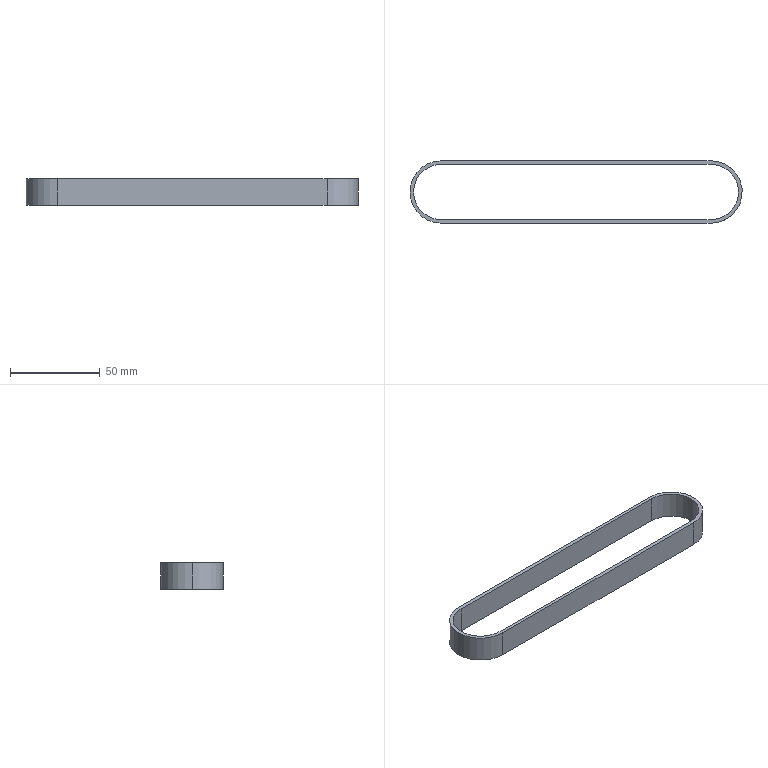Part | STEP file | HTBN400S5M-150 | 1 solid | 12 faces | box 185.61 x 34.88 x 15 mm | volume 12143 mm3 | cylinder 6 | plane 6 | commonest cylinder face diameters 30.88 x3 34.88 x3
STEP:
#1=CARTESIAN_POINT('',(0.,0.,0.));
#2=DIRECTION('',(0.,0.,1.));
#3=DIRECTION('',(1.,0.,0.));
#4=AXIS2_PLACEMENT_3D('',#1,#2,#3);
#5=CARTESIAN_POINT('',(-52.748,15.44,15.));
#6=VERTEX_POINT('',#5);
#7=CARTESIAN_POINT('',(-52.748,15.44,0.));
#8=VERTEX_POINT('',#7);
#9=CARTESIAN_POINT('',(-52.748,15.44,15.));
#10=DIRECTION('',(0.,0.,-1.));
#11=VECTOR('',#10,1.);
#12=LINE('',#9,#11);
#13=CARTESIAN_POINT('',(-52.748,0.,15.));
#14=DIRECTION('',(0.,0.,-1.));
#15=DIRECTION('',(-1.,0.,0.));
#16=AXIS2_PLACEMENT_3D('',#13,#14,#15);
#17=CYLINDRICAL_SURFACE('',#16,15.44);
#18=CARTESIAN_POINT('',(1.571,0.));
#19=DIRECTION('',(0.,1.));
#20=VECTOR('',#19,1.);
#21=LINE('',#18,#20);
#22=(GEOMETRIC_REPRESENTATION_CONTEXT(2)PARAMETRIC_REPRESENTATION_CONTEXT()REPRESENTATION_CONTEXT('',''));
#23=DEFINITIONAL_REPRESENTATION('',(#21),#22);
#24=PCURVE('',#17,#23);
#25=CARTESIAN_POINT('',(-52.748,15.44,15.));
#26=DIRECTION('',(0.,-1.,0.));
#27=DIRECTION('',(0.,0.,-1.));
#28=AXIS2_PLACEMENT_3D('',#25,#26,#27);
#29=PLANE('',#28);
#30=CARTESIAN_POINT('',(0.,0.));
#31=DIRECTION('',(1.,0.));
#32=VECTOR('',#31,1.);
#33=LINE('',#30,#32);
#34=(GEOMETRIC_REPRESENTATION_CONTEXT(2)PARAMETRIC_REPRESENTATION_CONTEXT()REPRESENTATION_CONTEXT('',''));
#35=DEFINITIONAL_REPRESENTATION('',(#33),#34);
#36=PCURVE('',#29,#35);
#37=SURFACE_CURVE('',#12,(#24,#36),.PCURVE_S1.);
#38=EDGE_CURVE('',#6,#8,#37,.T.);
#39=ORIENTED_EDGE('',*,*,#38,.T.);
#40=CARTESIAN_POINT('',(-68.188,0.,0.));
#41=VERTEX_POINT('',#40);
#42=CARTESIAN_POINT('',(-52.748,0.,0.));
#43=DIRECTION('',(0.,0.,1.));
#44=DIRECTION('',(1.,0.,0.));
#45=AXIS2_PLACEMENT_3D('',#42,#43,#44);
#46=CIRCLE('',#45,15.44);
#47=CARTESIAN_POINT('',(3.142,15.));
#48=DIRECTION('',(-1.,0.));
#49=VECTOR('',#48,1.);
#50=LINE('',#47,#49);
#51=(GEOMETRIC_REPRESENTATION_CONTEXT(2)PARAMETRIC_REPRESENTATION_CONTEXT()REPRESENTATION_CONTEXT('',''));
#52=DEFINITIONAL_REPRESENTATION('',(#50),#51);
#53=PCURVE('',#17,#52);
#54=CARTESIAN_POINT('',(-52.748,0.,0.));
#55=DIRECTION('',(0.,0.,1.));
#56=DIRECTION('',(1.,0.,0.));
#57=AXIS2_PLACEMENT_3D('',#54,#55,#56);
#58=PLANE('',#57);
#59=CARTESIAN_POINT('',(0.,0.));
#60=DIRECTION('',(1.,0.));
#61=AXIS2_PLACEMENT_2D('',#59,#60);
#62=CIRCLE('',#61,15.44);
#63=(GEOMETRIC_REPRESENTATION_CONTEXT(2)PARAMETRIC_REPRESENTATION_CONTEXT()REPRESENTATION_CONTEXT('',''));
#64=DEFINITIONAL_REPRESENTATION('',(#62),#63);
#65=PCURVE('',#58,#64);
#66=SURFACE_CURVE('',#46,(#53,#65),.PCURVE_S1.);
#67=EDGE_CURVE('',#8,#41,#66,.T.);
#68=ORIENTED_EDGE('',*,*,#67,.T.);
#69=CARTESIAN_POINT('',(-68.188,0.,15.));
#70=VERTEX_POINT('',#69);
#71=CARTESIAN_POINT('',(-68.188,0.,15.));
#72=DIRECTION('',(0.,0.,-1.));
#73=VECTOR('',#72,1.);
#74=LINE('',#71,#73);
#75=CARTESIAN_POINT('',(0.,0.));
#76=DIRECTION('',(0.,1.));
#77=VECTOR('',#76,1.);
#78=LINE('',#75,#77);
#79=(GEOMETRIC_REPRESENTATION_CONTEXT(2)PARAMETRIC_REPRESENTATION_CONTEXT()REPRESENTATION_CONTEXT('',''));
#80=DEFINITIONAL_REPRESENTATION('',(#78),#79);
#81=PCURVE('',#17,#80);
#82=CARTESIAN_POINT('',(-52.748,0.,15.));
#83=DIRECTION('',(0.,0.,-1.));
#84=DIRECTION('',(-1.,0.,0.));
#85=AXIS2_PLACEMENT_3D('',#82,#83,#84);
#86=CYLINDRICAL_SURFACE('',#85,15.44);
#87=CARTESIAN_POINT('',(6.283,0.));
#88=DIRECTION('',(0.,1.));
#89=VECTOR('',#88,1.);
#90=LINE('',#87,#89);
#91=(GEOMETRIC_REPRESENTATION_CONTEXT(2)PARAMETRIC_REPRESENTATION_CONTEXT()REPRESENTATION_CONTEXT('',''));
#92=DEFINITIONAL_REPRESENTATION('',(#90),#91);
#93=PCURVE('',#86,#92);
#94=SURFACE_CURVE('',#74,(#81,#93),.PCURVE_S1.);
#95=EDGE_CURVE('',#70,#41,#94,.T.);
#96=ORIENTED_EDGE('',*,*,#95,.F.);
#97=CARTESIAN_POINT('',(-52.748,0.,15.));
#98=DIRECTION('',(0.,0.,1.));
#99=DIRECTION('',(1.,0.,0.));
#100=AXIS2_PLACEMENT_3D('',#97,#98,#99);
#101=CIRCLE('',#100,15.44);
#102=CARTESIAN_POINT('',(3.142,0.));
#103=DIRECTION('',(-1.,0.));
#104=VECTOR('',#103,1.);
#105=LINE('',#102,#104);
#106=(GEOMETRIC_REPRESENTATION_CONTEXT(2)PARAMETRIC_REPRESENTATION_CONTEXT()REPRESENTATION_CONTEXT('',''));
#107=DEFINITIONAL_REPRESENTATION('',(#105),#106);
#108=PCURVE('',#17,#107);
#109=CARTESIAN_POINT('',(-52.748,0.,15.));
#110=DIRECTION('',(0.,0.,1.));
#111=DIRECTION('',(1.,0.,0.));
#112=AXIS2_PLACEMENT_3D('',#109,#110,#111);
#113=PLANE('',#112);
#114=CARTESIAN_POINT('',(0.,0.));
#115=DIRECTION('',(1.,0.));
#116=AXIS2_PLACEMENT_2D('',#114,#115);
#117=CIRCLE('',#116,15.44);
#118=(GEOMETRIC_REPRESENTATION_CONTEXT(2)PARAMETRIC_REPRESENTATION_CONTEXT()REPRESENTATION_CONTEXT('',''));
#119=DEFINITIONAL_REPRESENTATION('',(#117),#118);
#120=PCURVE('',#113,#119);
#121=SURFACE_CURVE('',#101,(#108,#120),.PCURVE_S1.);
#122=EDGE_CURVE('',#6,#70,#121,.T.);
#123=ORIENTED_EDGE('',*,*,#122,.F.);
#124=EDGE_LOOP('',(#39,#68,#96,#123));
#125=FACE_BOUND('',#124,.F.);
#126=ADVANCED_FACE('',(#125),#17,.F.);
#127=CARTESIAN_POINT('',(-70.188,0.,15.));
#128=VERTEX_POINT('',#127);
#129=CARTESIAN_POINT('',(-52.748,-17.44,15.));
#130=VERTEX_POINT('',#129);
#131=CARTESIAN_POINT('',(-52.748,0.,15.));
#132=DIRECTION('',(0.,0.,1.));
#133=DIRECTION('',(1.,0.,0.));
#134=AXIS2_PLACEMENT_3D('',#131,#132,#133);
#135=CIRCLE('',#134,17.44);
#136=CARTESIAN_POINT('',(-52.748,0.,15.));
#137=DIRECTION('',(0.,0.,-1.));
#138=DIRECTION('',(-1.,0.,0.));
#139=AXIS2_PLACEMENT_3D('',#136,#137,#138);
#140=CYLINDRICAL_SURFACE('',#139,17.44);
#141=CARTESIAN_POINT('',(9.425,0.));
#142=DIRECTION('',(-1.,0.));
#143=VECTOR('',#142,1.);
#144=LINE('',#141,#143);
#145=(GEOMETRIC_REPRESENTATION_CONTEXT(2)PARAMETRIC_REPRESENTATION_CONTEXT()REPRESENTATION_CONTEXT('',''));
#146=DEFINITIONAL_REPRESENTATION('',(#144),#145);
#147=PCURVE('',#140,#146);
#148=CARTESIAN_POINT('',(0.,0.));
#149=DIRECTION('',(1.,0.));
#150=AXIS2_PLACEMENT_2D('',#148,#149);
#151=CIRCLE('',#150,17.44);
#152=(GEOMETRIC_REPRESENTATION_CONTEXT(2)PARAMETRIC_REPRESENTATION_CONTEXT()REPRESENTATION_CONTEXT('',''));
#153=DEFINITIONAL_REPRESENTATION('',(#151),#152);
#154=PCURVE('',#113,#153);
#155=SURFACE_CURVE('',#135,(#147,#154),.PCURVE_S1.);
#156=EDGE_CURVE('',#128,#130,#155,.T.);
#157=ORIENTED_EDGE('',*,*,#156,.F.);
#158=CARTESIAN_POINT('',(-70.188,0.,0.));
#159=VERTEX_POINT('',#158);
#160=CARTESIAN_POINT('',(-70.188,0.,15.));
#161=DIRECTION('',(0.,0.,-1.));
#162=VECTOR('',#161,1.);
#163=LINE('',#160,#162);
#164=CARTESIAN_POINT('',(6.283,0.));
#165=DIRECTION('',(0.,1.));
#166=VECTOR('',#165,1.);
#167=LINE('',#164,#166);
#168=(GEOMETRIC_REPRESENTATION_CONTEXT(2)PARAMETRIC_REPRESENTATION_CONTEXT()REPRESENTATION_CONTEXT('',''));
#169=DEFINITIONAL_REPRESENTATION('',(#167),#168);
#170=PCURVE('',#140,#169);
#171=CARTESIAN_POINT('',(-52.748,0.,15.));
#172=DIRECTION('',(0.,0.,-1.));
#173=DIRECTION('',(-1.,0.,0.));
#174=AXIS2_PLACEMENT_3D('',#171,#172,#173);
#175=CYLINDRICAL_SURFACE('',#174,17.44);
#176=CARTESIAN_POINT('',(0.,0.));
#177=DIRECTION('',(0.,1.));
#178=VECTOR('',#177,1.);
#179=LINE('',#176,#178);
#180=(GEOMETRIC_REPRESENTATION_CONTEXT(2)PARAMETRIC_REPRESENTATION_CONTEXT()REPRESENTATION_CONTEXT('',''));
#181=DEFINITIONAL_REPRESENTATION('',(#179),#180);
#182=PCURVE('',#175,#181);
#183=SURFACE_CURVE('',#163,(#170,#182),.PCURVE_S1.);
#184=EDGE_CURVE('',#128,#159,#183,.T.);
#185=ORIENTED_EDGE('',*,*,#184,.T.);
#186=CARTESIAN_POINT('',(-52.748,-17.44,0.));
#187=VERTEX_POINT('',#186);
#188=CARTESIAN_POINT('',(-52.748,0.,0.));
#189=DIRECTION('',(0.,0.,1.));
#190=DIRECTION('',(1.,0.,0.));
#191=AXIS2_PLACEMENT_3D('',#188,#189,#190);
#192=CIRCLE('',#191,17.44);
#193=CARTESIAN_POINT('',(9.425,15.));
#194=DIRECTION('',(-1.,0.));
#195=VECTOR('',#194,1.);
#196=LINE('',#193,#195);
#197=(GEOMETRIC_REPRESENTATION_CONTEXT(2)PARAMETRIC_REPRESENTATION_CONTEXT()REPRESENTATION_CONTEXT('',''));
#198=DEFINITIONAL_REPRESENTATION('',(#196),#197);
#199=PCURVE('',#140,#198);
#200=CARTESIAN_POINT('',(0.,0.));
#201=DIRECTION('',(1.,0.));
#202=AXIS2_PLACEMENT_2D('',#200,#201);
#203=CIRCLE('',#202,17.44);
#204=(GEOMETRIC_REPRESENTATION_CONTEXT(2)PARAMETRIC_REPRESENTATION_CONTEXT()REPRESENTATION_CONTEXT('',''));
#205=DEFINITIONAL_REPRESENTATION('',(#203),#204);
#206=PCURVE('',#58,#205);
#207=SURFACE_CURVE('',#192,(#199,#206),.PCURVE_S1.);
#208=EDGE_CURVE('',#159,#187,#207,.T.);
#209=ORIENTED_EDGE('',*,*,#208,.T.);
#210=CARTESIAN_POINT('',(-52.748,-17.44,15.));
#211=DIRECTION('',(0.,0.,-1.));
#212=VECTOR('',#211,1.);
#213=LINE('',#210,#212);
#214=CARTESIAN_POINT('',(4.712,0.));
#215=DIRECTION('',(0.,1.));
#216=VECTOR('',#215,1.);
#217=LINE('',#214,#216);
#218=(GEOMETRIC_REPRESENTATION_CONTEXT(2)PARAMETRIC_REPRESENTATION_CONTEXT()REPRESENTATION_CONTEXT('',''));
#219=DEFINITIONAL_REPRESENTATION('',(#217),#218);
#220=PCURVE('',#140,#219);
#221=CARTESIAN_POINT('',(-52.748,-17.44,15.));
#222=DIRECTION('',(0.,1.,0.));
#223=DIRECTION('',(0.,0.,1.));
#224=AXIS2_PLACEMENT_3D('',#221,#222,#223);
#225=PLANE('',#224);
#226=CARTESIAN_POINT('',(0.,0.));
#227=DIRECTION('',(-1.,0.));
#228=VECTOR('',#227,1.);
#229=LINE('',#226,#228);
#230=(GEOMETRIC_REPRESENTATION_CONTEXT(2)PARAMETRIC_REPRESENTATION_CONTEXT()REPRESENTATION_CONTEXT('',''));
#231=DEFINITIONAL_REPRESENTATION('',(#229),#230);
#232=PCURVE('',#225,#231);
#233=SURFACE_CURVE('',#213,(#220,#232),.PCURVE_S1.);
#234=EDGE_CURVE('',#130,#187,#233,.T.);
#235=ORIENTED_EDGE('',*,*,#234,.F.);
#236=EDGE_LOOP('',(#157,#185,#209,#235));
#237=FACE_BOUND('',#236,.T.);
#238=ADVANCED_FACE('',(#237),#140,.T.);
#239=CARTESIAN_POINT('',(-52.748,17.44,15.));
#240=VERTEX_POINT('',#239);
#241=CARTESIAN_POINT('',(-52.748,0.,15.));
#242=DIRECTION('',(0.,0.,1.));
#243=DIRECTION('',(1.,0.,0.));
#244=AXIS2_PLACEMENT_3D('',#241,#242,#243);
#245=CIRCLE('',#244,17.44);
#246=CARTESIAN_POINT('',(0.,0.));
#247=DIRECTION('',(1.,0.));
#248=AXIS2_PLACEMENT_2D('',#246,#247);
#249=CIRCLE('',#248,17.44);
#250=(GEOMETRIC_REPRESENTATION_CONTEXT(2)PARAMETRIC_REPRESENTATION_CONTEXT()REPRESENTATION_CONTEXT('',''));
#251=DEFINITIONAL_REPRESENTATION('',(#249),#250);
#252=PCURVE('',#113,#251);
#253=CARTESIAN_POINT('',(3.142,0.));
#254=DIRECTION('',(-1.,0.));
#255=VECTOR('',#254,1.);
#256=LINE('',#253,#255);
#257=(GEOMETRIC_REPRESENTATION_CONTEXT(2)PARAMETRIC_REPRESENTATION_CONTEXT()REPRESENTATION_CONTEXT('',''));
#258=DEFINITIONAL_REPRESENTATION('',(#256),#257);
#259=PCURVE('',#175,#258);
#260=SURFACE_CURVE('',#245,(#252,#259),.PCURVE_S1.);
#261=EDGE_CURVE('',#240,#128,#260,.T.);
#262=ORIENTED_EDGE('',*,*,#261,.T.);
#263=ORIENTED_EDGE('',*,*,#156,.T.);
#264=CARTESIAN_POINT('',(97.982,-17.44,15.));
#265=VERTEX_POINT('',#264);
#266=CARTESIAN_POINT('',(-52.748,-17.44,15.));
#267=DIRECTION('',(1.,0.,0.));
#268=VECTOR('',#267,1.);
#269=LINE('',#266,#268);
#270=CARTESIAN_POINT('',(0.,-17.44));
#271=DIRECTION('',(1.,0.));
#272=VECTOR('',#271,1.);
#273=LINE('',#270,#272);
#274=(GEOMETRIC_REPRESENTATION_CONTEXT(2)PARAMETRIC_REPRESENTATION_CONTEXT()REPRESENTATION_CONTEXT('',''));
#275=DEFINITIONAL_REPRESENTATION('',(#273),#274);
#276=PCURVE('',#113,#275);
#277=CARTESIAN_POINT('',(0.,0.));
#278=DIRECTION('',(0.,1.));
#279=VECTOR('',#278,1.);
#280=LINE('',#277,#279);
#281=(GEOMETRIC_REPRESENTATION_CONTEXT(2)PARAMETRIC_REPRESENTATION_CONTEXT()REPRESENTATION_CONTEXT('',''));
#282=DEFINITIONAL_REPRESENTATION('',(#280),#281);
#283=PCURVE('',#225,#282);
#284=SURFACE_CURVE('',#269,(#276,#283),.PCURVE_S1.);
#285=EDGE_CURVE('',#130,#265,#284,.T.);
#286=ORIENTED_EDGE('',*,*,#285,.T.);
#287=CARTESIAN_POINT('',(97.982,17.44,15.));
#288=VERTEX_POINT('',#287);
#289=CARTESIAN_POINT('',(97.982,0.,15.));
#290=DIRECTION('',(0.,0.,1.));
#291=DIRECTION('',(1.,0.,0.));
#292=AXIS2_PLACEMENT_3D('',#289,#290,#291);
#293=CIRCLE('',#292,17.44);
#294=CARTESIAN_POINT('',(150.73,0.));
#295=DIRECTION('',(1.,0.));
#296=AXIS2_PLACEMENT_2D('',#294,#295);
#297=CIRCLE('',#296,17.44);
#298=(GEOMETRIC_REPRESENTATION_CONTEXT(2)PARAMETRIC_REPRESENTATION_CONTEXT()REPRESENTATION_CONTEXT('',''));
#299=DEFINITIONAL_REPRESENTATION('',(#297),#298);
#300=PCURVE('',#113,#299);
#301=CARTESIAN_POINT('',(97.982,0.,15.));
#302=DIRECTION('',(0.,0.,-1.));
#303=DIRECTION('',(-1.,0.,0.));
#304=AXIS2_PLACEMENT_3D('',#301,#302,#303);
#305=CYLINDRICAL_SURFACE('',#304,17.44);
#306=CARTESIAN_POINT('',(9.425,0.));
#307=DIRECTION('',(-1.,0.));
#308=VECTOR('',#307,1.);
#309=LINE('',#306,#308);
#310=(GEOMETRIC_REPRESENTATION_CONTEXT(2)PARAMETRIC_REPRESENTATION_CONTEXT()REPRESENTATION_CONTEXT('',''));
#311=DEFINITIONAL_REPRESENTATION('',(#309),#310);
#312=PCURVE('',#305,#311);
#313=SURFACE_CURVE('',#293,(#300,#312),.PCURVE_S1.);
#314=EDGE_CURVE('',#265,#288,#313,.T.);
#315=ORIENTED_EDGE('',*,*,#314,.T.);
#316=CARTESIAN_POINT('',(-52.748,17.44,15.));
#317=DIRECTION('',(-1.,0.,0.));
#318=VECTOR('',#317,1.);
#319=LINE('',#316,#318);
#320=CARTESIAN_POINT('',(0.,17.44));
#321=DIRECTION('',(-1.,0.));
#322=VECTOR('',#321,1.);
#323=LINE('',#320,#322);
#324=(GEOMETRIC_REPRESENTATION_CONTEXT(2)PARAMETRIC_REPRESENTATION_CONTEXT()REPRESENTATION_CONTEXT('',''));
#325=DEFINITIONAL_REPRESENTATION('',(#323),#324);
#326=PCURVE('',#113,#325);
#327=CARTESIAN_POINT('',(-52.748,17.44,15.));
#328=DIRECTION('',(0.,-1.,0.));
#329=DIRECTION('',(0.,0.,-1.));
#330=AXIS2_PLACEMENT_3D('',#327,#328,#329);
#331=PLANE('',#330);
#332=CARTESIAN_POINT('',(0.,0.));
#333=DIRECTION('',(0.,-1.));
#334=VECTOR('',#333,1.);
#335=LINE('',#332,#334);
#336=(GEOMETRIC_REPRESENTATION_CONTEXT(2)PARAMETRIC_REPRESENTATION_CONTEXT()REPRESENTATION_CONTEXT('',''));
#337=DEFINITIONAL_REPRESENTATION('',(#335),#336);
#338=PCURVE('',#331,#337);
#339=SURFACE_CURVE('',#319,(#326,#338),.PCURVE_S1.);
#340=EDGE_CURVE('',#288,#240,#339,.T.);
#341=ORIENTED_EDGE('',*,*,#340,.T.);
#342=EDGE_LOOP('',(#262,#263,#286,#315,#341));
#343=FACE_BOUND('',#342,.T.);
#344=CARTESIAN_POINT('',(-52.748,-15.44,15.));
#345=VERTEX_POINT('',#344);
#346=CARTESIAN_POINT('',(97.982,-15.44,15.));
#347=VERTEX_POINT('',#346);
#348=CARTESIAN_POINT('',(-52.748,-15.44,15.));
#349=DIRECTION('',(1.,0.,0.));
#350=VECTOR('',#349,1.);
#351=LINE('',#348,#350);
#352=CARTESIAN_POINT('',(0.,-15.44));
#353=DIRECTION('',(1.,0.));
#354=VECTOR('',#353,1.);
#355=LINE('',#352,#354);
#356=(GEOMETRIC_REPRESENTATION_CONTEXT(2)PARAMETRIC_REPRESENTATION_CONTEXT()REPRESENTATION_CONTEXT('',''));
#357=DEFINITIONAL_REPRESENTATION('',(#355),#356);
#358=PCURVE('',#113,#357);
#359=CARTESIAN_POINT('',(-52.748,-15.44,15.));
#360=DIRECTION('',(0.,1.,0.));
#361=DIRECTION('',(0.,0.,1.));
#362=AXIS2_PLACEMENT_3D('',#359,#360,#361);
#363=PLANE('',#362);
#364=CARTESIAN_POINT('',(0.,0.));
#365=DIRECTION('',(0.,1.));
#366=VECTOR('',#365,1.);
#367=LINE('',#364,#366);
#368=(GEOMETRIC_REPRESENTATION_CONTEXT(2)PARAMETRIC_REPRESENTATION_CONTEXT()REPRESENTATION_CONTEXT('',''));
#369=DEFINITIONAL_REPRESENTATION('',(#367),#368);
#370=PCURVE('',#363,#369);
#371=SURFACE_CURVE('',#351,(#358,#370),.PCURVE_S1.);
#372=EDGE_CURVE('',#345,#347,#371,.T.);
#373=ORIENTED_EDGE('',*,*,#372,.F.);
#374=CARTESIAN_POINT('',(-52.748,0.,15.));
#375=DIRECTION('',(0.,0.,1.));
#376=DIRECTION('',(1.,0.,0.));
#377=AXIS2_PLACEMENT_3D('',#374,#375,#376);
#378=CIRCLE('',#377,15.44);
#379=CARTESIAN_POINT('',(0.,0.));
#380=DIRECTION('',(1.,0.));
#381=AXIS2_PLACEMENT_2D('',#379,#380);
#382=CIRCLE('',#381,15.44);
#383=(GEOMETRIC_REPRESENTATION_CONTEXT(2)PARAMETRIC_REPRESENTATION_CONTEXT()REPRESENTATION_CONTEXT('',''));
#384=DEFINITIONAL_REPRESENTATION('',(#382),#383);
#385=PCURVE('',#113,#384);
#386=CARTESIAN_POINT('',(9.425,0.));
#387=DIRECTION('',(-1.,0.));
#388=VECTOR('',#387,1.);
#389=LINE('',#386,#388);
#390=(GEOMETRIC_REPRESENTATION_CONTEXT(2)PARAMETRIC_REPRESENTATION_CONTEXT()REPRESENTATION_CONTEXT('',''));
#391=DEFINITIONAL_REPRESENTATION('',(#389),#390);
#392=PCURVE('',#86,#391);
#393=SURFACE_CURVE('',#378,(#385,#392),.PCURVE_S1.);
#394=EDGE_CURVE('',#70,#345,#393,.T.);
#395=ORIENTED_EDGE('',*,*,#394,.F.);
#396=ORIENTED_EDGE('',*,*,#122,.F.);
#397=CARTESIAN_POINT('',(97.982,15.44,15.));
#398=VERTEX_POINT('',#397);
#399=CARTESIAN_POINT('',(-52.748,15.44,15.));
#400=DIRECTION('',(-1.,0.,0.));
#401=VECTOR('',#400,1.);
#402=LINE('',#399,#401);
#403=CARTESIAN_POINT('',(0.,15.44));
#404=DIRECTION('',(-1.,0.));
#405=VECTOR('',#404,1.);
#406=LINE('',#403,#405);
#407=(GEOMETRIC_REPRESENTATION_CONTEXT(2)PARAMETRIC_REPRESENTATION_CONTEXT()REPRESENTATION_CONTEXT('',''));
#408=DEFINITIONAL_REPRESENTATION('',(#406),#407);
#409=PCURVE('',#113,#408);
#410=CARTESIAN_POINT('',(0.,0.));
#411=DIRECTION('',(0.,-1.));
#412=VECTOR('',#411,1.);
#413=LINE('',#410,#412);
#414=(GEOMETRIC_REPRESENTATION_CONTEXT(2)PARAMETRIC_REPRESENTATION_CONTEXT()REPRESENTATION_CONTEXT('',''));
#415=DEFINITIONAL_REPRESENTATION('',(#413),#414);
#416=PCURVE('',#29,#415);
#417=SURFACE_CURVE('',#402,(#409,#416),.PCURVE_S1.);
#418=EDGE_CURVE('',#398,#6,#417,.T.);
#419=ORIENTED_EDGE('',*,*,#418,.F.);
#420=CARTESIAN_POINT('',(97.982,0.,15.));
#421=DIRECTION('',(0.,0.,1.));
#422=DIRECTION('',(1.,0.,0.));
#423=AXIS2_PLACEMENT_3D('',#420,#421,#422);
#424=CIRCLE('',#423,15.44);
#425=CARTESIAN_POINT('',(150.73,0.));
#426=DIRECTION('',(1.,0.));
#427=AXIS2_PLACEMENT_2D('',#425,#426);
#428=CIRCLE('',#427,15.44);
#429=(GEOMETRIC_REPRESENTATION_CONTEXT(2)PARAMETRIC_REPRESENTATION_CONTEXT()REPRESENTATION_CONTEXT('',''));
#430=DEFINITIONAL_REPRESENTATION('',(#428),#429);
#431=PCURVE('',#113,#430);
#432=CARTESIAN_POINT('',(97.982,0.,15.));
#433=DIRECTION('',(0.,0.,-1.));
#434=DIRECTION('',(-1.,0.,0.));
#435=AXIS2_PLACEMENT_3D('',#432,#433,#434);
#436=CYLINDRICAL_SURFACE('',#435,15.44);
#437=CARTESIAN_POINT('',(9.425,0.));
#438=DIRECTION('',(-1.,0.));
#439=VECTOR('',#438,1.);
#440=LINE('',#437,#439);
#441=(GEOMETRIC_REPRESENTATION_CONTEXT(2)PARAMETRIC_REPRESENTATION_CONTEXT()REPRESENTATION_CONTEXT('',''));
#442=DEFINITIONAL_REPRESENTATION('',(#440),#441);
#443=PCURVE('',#436,#442);
#444=SURFACE_CURVE('',#424,(#431,#443),.PCURVE_S1.);
#445=EDGE_CURVE('',#347,#398,#444,.T.);
#446=ORIENTED_EDGE('',*,*,#445,.F.);
#447=EDGE_LOOP('',(#373,#395,#396,#419,#446));
#448=FACE_BOUND('',#447,.T.);
#449=ADVANCED_FACE('',(#343,#448),#113,.T.);
#450=CARTESIAN_POINT('',(-52.748,17.44,0.));
#451=VERTEX_POINT('',#450);
#452=CARTESIAN_POINT('',(-52.748,0.,0.));
#453=DIRECTION('',(0.,0.,1.));
#454=DIRECTION('',(1.,0.,0.));
#455=AXIS2_PLACEMENT_3D('',#452,#453,#454);
#456=CIRCLE('',#455,17.44);
#457=CARTESIAN_POINT('',(0.,0.));
#458=DIRECTION('',(1.,0.));
#459=AXIS2_PLACEMENT_2D('',#457,#458);
#460=CIRCLE('',#459,17.44);
#461=(GEOMETRIC_REPRESENTATION_CONTEXT(2)PARAMETRIC_REPRESENTATION_CONTEXT()REPRESENTATION_CONTEXT('',''));
#462=DEFINITIONAL_REPRESENTATION('',(#460),#461);
#463=PCURVE('',#58,#462);
#464=CARTESIAN_POINT('',(3.142,15.));
#465=DIRECTION('',(-1.,0.));
#466=VECTOR('',#465,1.);
#467=LINE('',#464,#466);
#468=(GEOMETRIC_REPRESENTATION_CONTEXT(2)PARAMETRIC_REPRESENTATION_CONTEXT()REPRESENTATION_CONTEXT('',''));
#469=DEFINITIONAL_REPRESENTATION('',(#467),#468);
#470=PCURVE('',#175,#469);
#471=SURFACE_CURVE('',#456,(#463,#470),.PCURVE_S1.);
#472=EDGE_CURVE('',#451,#159,#471,.T.);
#473=ORIENTED_EDGE('',*,*,#472,.F.);
#474=CARTESIAN_POINT('',(97.982,17.44,0.));
#475=VERTEX_POINT('',#474);
#476=CARTESIAN_POINT('',(-52.748,17.44,0.));
#477=DIRECTION('',(-1.,0.,0.));
#478=VECTOR('',#477,1.);
#479=LINE('',#476,#478);
#480=CARTESIAN_POINT('',(0.,17.44));
#481=DIRECTION('',(-1.,0.));
#482=VECTOR('',#481,1.);
#483=LINE('',#480,#482);
#484=(GEOMETRIC_REPRESENTATION_CONTEXT(2)PARAMETRIC_REPRESENTATION_CONTEXT()REPRESENTATION_CONTEXT('',''));
#485=DEFINITIONAL_REPRESENTATION('',(#483),#484);
#486=PCURVE('',#58,#485);
#487=CARTESIAN_POINT('',(15.,0.));
#488=DIRECTION('',(0.,-1.));
#489=VECTOR('',#488,1.);
#490=LINE('',#487,#489);
#491=(GEOMETRIC_REPRESENTATION_CONTEXT(2)PARAMETRIC_REPRESENTATION_CONTEXT()REPRESENTATION_CONTEXT('',''));
#492=DEFINITIONAL_REPRESENTATION('',(#490),#491);
#493=PCURVE('',#331,#492);
#494=SURFACE_CURVE('',#479,(#486,#493),.PCURVE_S1.);
#495=EDGE_CURVE('',#475,#451,#494,.T.);
#496=ORIENTED_EDGE('',*,*,#495,.F.);
#497=CARTESIAN_POINT('',(97.982,-17.44,0.));
#498=VERTEX_POINT('',#497);
#499=CARTESIAN_POINT('',(97.982,0.,0.));
#500=DIRECTION('',(0.,0.,1.));
#501=DIRECTION('',(1.,0.,0.));
#502=AXIS2_PLACEMENT_3D('',#499,#500,#501);
#503=CIRCLE('',#502,17.44);
#504=CARTESIAN_POINT('',(150.73,0.));
#505=DIRECTION('',(1.,0.));
#506=AXIS2_PLACEMENT_2D('',#504,#505);
#507=CIRCLE('',#506,17.44);
#508=(GEOMETRIC_REPRESENTATION_CONTEXT(2)PARAMETRIC_REPRESENTATION_CONTEXT()REPRESENTATION_CONTEXT('',''));
#509=DEFINITIONAL_REPRESENTATION('',(#507),#508);
#510=PCURVE('',#58,#509);
#511=CARTESIAN_POINT('',(9.425,15.));
#512=DIRECTION('',(-1.,0.));
#513=VECTOR('',#512,1.);
#514=LINE('',#511,#513);
#515=(GEOMETRIC_REPRESENTATION_CONTEXT(2)PARAMETRIC_REPRESENTATION_CONTEXT()REPRESENTATION_CONTEXT('',''));
#516=DEFINITIONAL_REPRESENTATION('',(#514),#515);
#517=PCURVE('',#305,#516);
#518=SURFACE_CURVE('',#503,(#510,#517),.PCURVE_S1.);
#519=EDGE_CURVE('',#498,#475,#518,.T.);
#520=ORIENTED_EDGE('',*,*,#519,.F.);
#521=CARTESIAN_POINT('',(-52.748,-17.44,0.));
#522=DIRECTION('',(1.,0.,0.));
#523=VECTOR('',#522,1.);
#524=LINE('',#521,#523);
#525=CARTESIAN_POINT('',(0.,-17.44));
#526=DIRECTION('',(1.,0.));
#527=VECTOR('',#526,1.);
#528=LINE('',#525,#527);
#529=(GEOMETRIC_REPRESENTATION_CONTEXT(2)PARAMETRIC_REPRESENTATION_CONTEXT()REPRESENTATION_CONTEXT('',''));
#530=DEFINITIONAL_REPRESENTATION('',(#528),#529);
#531=PCURVE('',#58,#530);
#532=CARTESIAN_POINT('',(-15.,0.));
#533=DIRECTION('',(0.,1.));
#534=VECTOR('',#533,1.);
#535=LINE('',#532,#534);
#536=(GEOMETRIC_REPRESENTATION_CONTEXT(2)PARAMETRIC_REPRESENTATION_CONTEXT()REPRESENTATION_CONTEXT('',''));
#537=DEFINITIONAL_REPRESENTATION('',(#535),#536);
#538=PCURVE('',#225,#537);
#539=SURFACE_CURVE('',#524,(#531,#538),.PCURVE_S1.);
#540=EDGE_CURVE('',#187,#498,#539,.T.);
#541=ORIENTED_EDGE('',*,*,#540,.F.);
#542=ORIENTED_EDGE('',*,*,#208,.F.);
#543=EDGE_LOOP('',(#473,#496,#520,#541,#542));
#544=FACE_BOUND('',#543,.T.);
#545=ORIENTED_EDGE('',*,*,#67,.T.);
#546=CARTESIAN_POINT('',(-52.748,-15.44,0.));
#547=VERTEX_POINT('',#546);
#548=CARTESIAN_POINT('',(-52.748,0.,0.));
#549=DIRECTION('',(0.,0.,1.));
#550=DIRECTION('',(1.,0.,0.));
#551=AXIS2_PLACEMENT_3D('',#548,#549,#550);
#552=CIRCLE('',#551,15.44);
#553=CARTESIAN_POINT('',(0.,0.));
#554=DIRECTION('',(1.,0.));
#555=AXIS2_PLACEMENT_2D('',#553,#554);
#556=CIRCLE('',#555,15.44);
#557=(GEOMETRIC_REPRESENTATION_CONTEXT(2)PARAMETRIC_REPRESENTATION_CONTEXT()REPRESENTATION_CONTEXT('',''));
#558=DEFINITIONAL_REPRESENTATION('',(#556),#557);
#559=PCURVE('',#58,#558);
#560=CARTESIAN_POINT('',(9.425,15.));
#561=DIRECTION('',(-1.,0.));
#562=VECTOR('',#561,1.);
#563=LINE('',#560,#562);
#564=(GEOMETRIC_REPRESENTATION_CONTEXT(2)PARAMETRIC_REPRESENTATION_CONTEXT()REPRESENTATION_CONTEXT('',''));
#565=DEFINITIONAL_REPRESENTATION('',(#563),#564);
#566=PCURVE('',#86,#565);
#567=SURFACE_CURVE('',#552,(#559,#566),.PCURVE_S1.);
#568=EDGE_CURVE('',#41,#547,#567,.T.);
#569=ORIENTED_EDGE('',*,*,#568,.T.);
#570=CARTESIAN_POINT('',(97.982,-15.44,0.));
#571=VERTEX_POINT('',#570);
#572=CARTESIAN_POINT('',(-52.748,-15.44,0.));
#573=DIRECTION('',(1.,0.,0.));
#574=VECTOR('',#573,1.);
#575=LINE('',#572,#574);
#576=CARTESIAN_POINT('',(0.,-15.44));
#577=DIRECTION('',(1.,0.));
#578=VECTOR('',#577,1.);
#579=LINE('',#576,#578);
#580=(GEOMETRIC_REPRESENTATION_CONTEXT(2)PARAMETRIC_REPRESENTATION_CONTEXT()REPRESENTATION_CONTEXT('',''));
#581=DEFINITIONAL_REPRESENTATION('',(#579),#580);
#582=PCURVE('',#58,#581);
#583=CARTESIAN_POINT('',(-15.,0.));
#584=DIRECTION('',(0.,1.));
#585=VECTOR('',#584,1.);
#586=LINE('',#583,#585);
#587=(GEOMETRIC_REPRESENTATION_CONTEXT(2)PARAMETRIC_REPRESENTATION_CONTEXT()REPRESENTATION_CONTEXT('',''));
#588=DEFINITIONAL_REPRESENTATION('',(#586),#587);
#589=PCURVE('',#363,#588);
#590=SURFACE_CURVE('',#575,(#582,#589),.PCURVE_S1.);
#591=EDGE_CURVE('',#547,#571,#590,.T.);
#592=ORIENTED_EDGE('',*,*,#591,.T.);
#593=CARTESIAN_POINT('',(97.982,15.44,0.));
#594=VERTEX_POINT('',#593);
#595=CARTESIAN_POINT('',(97.982,0.,0.));
#596=DIRECTION('',(0.,0.,1.));
#597=DIRECTION('',(1.,0.,0.));
#598=AXIS2_PLACEMENT_3D('',#595,#596,#597);
#599=CIRCLE('',#598,15.44);
#600=CARTESIAN_POINT('',(150.73,0.));
#601=DIRECTION('',(1.,0.));
#602=AXIS2_PLACEMENT_2D('',#600,#601);
#603=CIRCLE('',#602,15.44);
#604=(GEOMETRIC_REPRESENTATION_CONTEXT(2)PARAMETRIC_REPRESENTATION_CONTEXT()REPRESENTATION_CONTEXT('',''));
#605=DEFINITIONAL_REPRESENTATION('',(#603),#604);
#606=PCURVE('',#58,#605);
#607=CARTESIAN_POINT('',(9.425,15.));
#608=DIRECTION('',(-1.,0.));
#609=VECTOR('',#608,1.);
#610=LINE('',#607,#609);
#611=(GEOMETRIC_REPRESENTATION_CONTEXT(2)PARAMETRIC_REPRESENTATION_CONTEXT()REPRESENTATION_CONTEXT('',''));
#612=DEFINITIONAL_REPRESENTATION('',(#610),#611);
#613=PCURVE('',#436,#612);
#614=SURFACE_CURVE('',#599,(#606,#613),.PCURVE_S1.);
#615=EDGE_CURVE('',#571,#594,#614,.T.);
#616=ORIENTED_EDGE('',*,*,#615,.T.);
#617=CARTESIAN_POINT('',(-52.748,15.44,0.));
#618=DIRECTION('',(-1.,0.,0.));
#619=VECTOR('',#618,1.);
#620=LINE('',#617,#619);
#621=CARTESIAN_POINT('',(0.,15.44));
#622=DIRECTION('',(-1.,0.));
#623=VECTOR('',#622,1.);
#624=LINE('',#621,#623);
#625=(GEOMETRIC_REPRESENTATION_CONTEXT(2)PARAMETRIC_REPRESENTATION_CONTEXT()REPRESENTATION_CONTEXT('',''));
#626=DEFINITIONAL_REPRESENTATION('',(#624),#625);
#627=PCURVE('',#58,#626);
#628=CARTESIAN_POINT('',(15.,0.));
#629=DIRECTION('',(0.,-1.));
#630=VECTOR('',#629,1.);
#631=LINE('',#628,#630);
#632=(GEOMETRIC_REPRESENTATION_CONTEXT(2)PARAMETRIC_REPRESENTATION_CONTEXT()REPRESENTATION_CONTEXT('',''));
#633=DEFINITIONAL_REPRESENTATION('',(#631),#632);
#634=PCURVE('',#29,#633);
#635=SURFACE_CURVE('',#620,(#627,#634),.PCURVE_S1.);
#636=EDGE_CURVE('',#594,#8,#635,.T.);
#637=ORIENTED_EDGE('',*,*,#636,.T.);
#638=EDGE_LOOP('',(#545,#569,#592,#616,#637));
#639=FACE_BOUND('',#638,.T.);
#640=ADVANCED_FACE('',(#544,#639),#58,.F.);
#641=ORIENTED_EDGE('',*,*,#184,.F.);
#642=ORIENTED_EDGE('',*,*,#261,.F.);
#643=CARTESIAN_POINT('',(-52.748,17.44,15.));
#644=DIRECTION('',(0.,0.,-1.));
#645=VECTOR('',#644,1.);
#646=LINE('',#643,#645);
#647=CARTESIAN_POINT('',(1.571,0.));
#648=DIRECTION('',(0.,1.));
#649=VECTOR('',#648,1.);
#650=LINE('',#647,#649);
#651=(GEOMETRIC_REPRESENTATION_CONTEXT(2)PARAMETRIC_REPRESENTATION_CONTEXT()REPRESENTATION_CONTEXT('',''));
#652=DEFINITIONAL_REPRESENTATION('',(#650),#651);
#653=PCURVE('',#175,#652);
#654=CARTESIAN_POINT('',(0.,0.));
#655=DIRECTION('',(1.,0.));
#656=VECTOR('',#655,1.);
#657=LINE('',#654,#656);
#658=(GEOMETRIC_REPRESENTATION_CONTEXT(2)PARAMETRIC_REPRESENTATION_CONTEXT()REPRESENTATION_CONTEXT('',''));
#659=DEFINITIONAL_REPRESENTATION('',(#657),#658);
#660=PCURVE('',#331,#659);
#661=SURFACE_CURVE('',#646,(#653,#660),.PCURVE_S1.);
#662=EDGE_CURVE('',#240,#451,#661,.T.);
#663=ORIENTED_EDGE('',*,*,#662,.T.);
#664=ORIENTED_EDGE('',*,*,#472,.T.);
#665=EDGE_LOOP('',(#641,#642,#663,#664));
#666=FACE_BOUND('',#665,.T.);
#667=ADVANCED_FACE('',(#666),#175,.T.);
#668=ORIENTED_EDGE('',*,*,#540,.T.);
#669=CARTESIAN_POINT('',(97.982,-17.44,15.));
#670=DIRECTION('',(0.,0.,-1.));
#671=VECTOR('',#670,1.);
#672=LINE('',#669,#671);
#673=CARTESIAN_POINT('',(0.,150.73));
#674=DIRECTION('',(-1.,0.));
#675=VECTOR('',#674,1.);
#676=LINE('',#673,#675);
#677=(GEOMETRIC_REPRESENTATION_CONTEXT(2)PARAMETRIC_REPRESENTATION_CONTEXT()REPRESENTATION_CONTEXT('',''));
#678=DEFINITIONAL_REPRESENTATION('',(#676),#677);
#679=PCURVE('',#225,#678);
#680=CARTESIAN_POINT('',(4.712,0.));
#681=DIRECTION('',(0.,1.));
#682=VECTOR('',#681,1.);
#683=LINE('',#680,#682);
#684=(GEOMETRIC_REPRESENTATION_CONTEXT(2)PARAMETRIC_REPRESENTATION_CONTEXT()REPRESENTATION_CONTEXT('',''));
#685=DEFINITIONAL_REPRESENTATION('',(#683),#684);
#686=PCURVE('',#305,#685);
#687=SURFACE_CURVE('',#672,(#679,#686),.PCURVE_S1.);
#688=EDGE_CURVE('',#265,#498,#687,.T.);
#689=ORIENTED_EDGE('',*,*,#688,.F.);
#690=ORIENTED_EDGE('',*,*,#285,.F.);
#691=ORIENTED_EDGE('',*,*,#234,.T.);
#692=EDGE_LOOP('',(#668,#689,#690,#691));
#693=FACE_BOUND('',#692,.T.);
#694=ADVANCED_FACE('',(#693),#225,.F.);
#695=ORIENTED_EDGE('',*,*,#519,.T.);
#696=CARTESIAN_POINT('',(97.982,17.44,15.));
#697=DIRECTION('',(0.,0.,-1.));
#698=VECTOR('',#697,1.);
#699=LINE('',#696,#698);
#700=CARTESIAN_POINT('',(1.571,0.));
#701=DIRECTION('',(0.,1.));
#702=VECTOR('',#701,1.);
#703=LINE('',#700,#702);
#704=(GEOMETRIC_REPRESENTATION_CONTEXT(2)PARAMETRIC_REPRESENTATION_CONTEXT()REPRESENTATION_CONTEXT('',''));
#705=DEFINITIONAL_REPRESENTATION('',(#703),#704);
#706=PCURVE('',#305,#705);
#707=CARTESIAN_POINT('',(0.,150.73));
#708=DIRECTION('',(1.,0.));
#709=VECTOR('',#708,1.);
#710=LINE('',#707,#709);
#711=(GEOMETRIC_REPRESENTATION_CONTEXT(2)PARAMETRIC_REPRESENTATION_CONTEXT()REPRESENTATION_CONTEXT('',''));
#712=DEFINITIONAL_REPRESENTATION('',(#710),#711);
#713=PCURVE('',#331,#712);
#714=SURFACE_CURVE('',#699,(#706,#713),.PCURVE_S1.);
#715=EDGE_CURVE('',#288,#475,#714,.T.);
#716=ORIENTED_EDGE('',*,*,#715,.F.);
#717=ORIENTED_EDGE('',*,*,#314,.F.);
#718=ORIENTED_EDGE('',*,*,#688,.T.);
#719=EDGE_LOOP('',(#695,#716,#717,#718));
#720=FACE_BOUND('',#719,.T.);
#721=ADVANCED_FACE('',(#720),#305,.T.);
#722=ORIENTED_EDGE('',*,*,#495,.T.);
#723=ORIENTED_EDGE('',*,*,#662,.F.);
#724=ORIENTED_EDGE('',*,*,#340,.F.);
#725=ORIENTED_EDGE('',*,*,#715,.T.);
#726=EDGE_LOOP('',(#722,#723,#724,#725));
#727=FACE_BOUND('',#726,.T.);
#728=ADVANCED_FACE('',(#727),#331,.F.);
#729=ORIENTED_EDGE('',*,*,#568,.T.);
#730=CARTESIAN_POINT('',(-52.748,-15.44,15.));
#731=DIRECTION('',(0.,0.,-1.));
#732=VECTOR('',#731,1.);
#733=LINE('',#730,#732);
#734=CARTESIAN_POINT('',(4.712,0.));
#735=DIRECTION('',(0.,1.));
#736=VECTOR('',#735,1.);
#737=LINE('',#734,#736);
#738=(GEOMETRIC_REPRESENTATION_CONTEXT(2)PARAMETRIC_REPRESENTATION_CONTEXT()REPRESENTATION_CONTEXT('',''));
#739=DEFINITIONAL_REPRESENTATION('',(#737),#738);
#740=PCURVE('',#86,#739);
#741=CARTESIAN_POINT('',(0.,0.));
#742=DIRECTION('',(-1.,0.));
#743=VECTOR('',#742,1.);
#744=LINE('',#741,#743);
#745=(GEOMETRIC_REPRESENTATION_CONTEXT(2)PARAMETRIC_REPRESENTATION_CONTEXT()REPRESENTATION_CONTEXT('',''));
#746=DEFINITIONAL_REPRESENTATION('',(#744),#745);
#747=PCURVE('',#363,#746);
#748=SURFACE_CURVE('',#733,(#740,#747),.PCURVE_S1.);
#749=EDGE_CURVE('',#345,#547,#748,.T.);
#750=ORIENTED_EDGE('',*,*,#749,.F.);
#751=ORIENTED_EDGE('',*,*,#394,.F.);
#752=ORIENTED_EDGE('',*,*,#95,.T.);
#753=EDGE_LOOP('',(#729,#750,#751,#752));
#754=FACE_BOUND('',#753,.F.);
#755=ADVANCED_FACE('',(#754),#86,.F.);
#756=ORIENTED_EDGE('',*,*,#591,.F.);
#757=ORIENTED_EDGE('',*,*,#749,.F.);
#758=ORIENTED_EDGE('',*,*,#372,.T.);
#759=CARTESIAN_POINT('',(97.982,-15.44,15.));
#760=DIRECTION('',(0.,0.,-1.));
#761=VECTOR('',#760,1.);
#762=LINE('',#759,#761);
#763=CARTESIAN_POINT('',(0.,150.73));
#764=DIRECTION('',(-1.,0.));
#765=VECTOR('',#764,1.);
#766=LINE('',#763,#765);
#767=(GEOMETRIC_REPRESENTATION_CONTEXT(2)PARAMETRIC_REPRESENTATION_CONTEXT()REPRESENTATION_CONTEXT('',''));
#768=DEFINITIONAL_REPRESENTATION('',(#766),#767);
#769=PCURVE('',#363,#768);
#770=CARTESIAN_POINT('',(4.712,0.));
#771=DIRECTION('',(0.,1.));
#772=VECTOR('',#771,1.);
#773=LINE('',#770,#772);
#774=(GEOMETRIC_REPRESENTATION_CONTEXT(2)PARAMETRIC_REPRESENTATION_CONTEXT()REPRESENTATION_CONTEXT('',''));
#775=DEFINITIONAL_REPRESENTATION('',(#773),#774);
#776=PCURVE('',#436,#775);
#777=SURFACE_CURVE('',#762,(#769,#776),.PCURVE_S1.);
#778=EDGE_CURVE('',#347,#571,#777,.T.);
#779=ORIENTED_EDGE('',*,*,#778,.T.);
#780=EDGE_LOOP('',(#756,#757,#758,#779));
#781=FACE_BOUND('',#780,.T.);
#782=ADVANCED_FACE('',(#781),#363,.T.);
#783=CARTESIAN_POINT('',(97.982,15.44,15.));
#784=DIRECTION('',(0.,0.,-1.));
#785=VECTOR('',#784,1.);
#786=LINE('',#783,#785);
#787=CARTESIAN_POINT('',(1.571,0.));
#788=DIRECTION('',(0.,1.));
#789=VECTOR('',#788,1.);
#790=LINE('',#787,#789);
#791=(GEOMETRIC_REPRESENTATION_CONTEXT(2)PARAMETRIC_REPRESENTATION_CONTEXT()REPRESENTATION_CONTEXT('',''));
#792=DEFINITIONAL_REPRESENTATION('',(#790),#791);
#793=PCURVE('',#436,#792);
#794=CARTESIAN_POINT('',(0.,150.73));
#795=DIRECTION('',(1.,0.));
#796=VECTOR('',#795,1.);
#797=LINE('',#794,#796);
#798=(GEOMETRIC_REPRESENTATION_CONTEXT(2)PARAMETRIC_REPRESENTATION_CONTEXT()REPRESENTATION_CONTEXT('',''));
#799=DEFINITIONAL_REPRESENTATION('',(#797),#798);
#800=PCURVE('',#29,#799);
#801=SURFACE_CURVE('',#786,(#793,#800),.PCURVE_S1.);
#802=EDGE_CURVE('',#398,#594,#801,.T.);
#803=ORIENTED_EDGE('',*,*,#802,.F.);
#804=ORIENTED_EDGE('',*,*,#445,.F.);
#805=ORIENTED_EDGE('',*,*,#778,.T.);
#806=ORIENTED_EDGE('',*,*,#615,.T.);
#807=EDGE_LOOP('',(#803,#804,#805,#806));
#808=FACE_BOUND('',#807,.F.);
#809=ADVANCED_FACE('',(#808),#436,.F.);
#810=ORIENTED_EDGE('',*,*,#636,.F.);
#811=ORIENTED_EDGE('',*,*,#802,.F.);
#812=ORIENTED_EDGE('',*,*,#418,.T.);
#813=ORIENTED_EDGE('',*,*,#38,.T.);
#814=EDGE_LOOP('',(#810,#811,#812,#813));
#815=FACE_BOUND('',#814,.T.);
#816=ADVANCED_FACE('',(#815),#29,.T.);
#817=CLOSED_SHELL('',(#126,#238,#449,#640,#667,#694,#721,#728,#755,#782,#809,#816));
#818=MANIFOLD_SOLID_BREP('',#817);
#819=(LENGTH_UNIT()NAMED_UNIT(*)SI_UNIT(.MILLI.,.METRE.));
#820=UNCERTAINTY_MEASURE_WITH_UNIT(LENGTH_MEASURE(0.0000001),#819,'','');
#821=(NAMED_UNIT(*)PLANE_ANGLE_UNIT()SI_UNIT($,.RADIAN.));
#822=(NAMED_UNIT(*)SI_UNIT($,.STERADIAN.)SOLID_ANGLE_UNIT());
#823=(GEOMETRIC_REPRESENTATION_CONTEXT(3)GLOBAL_UNCERTAINTY_ASSIGNED_CONTEXT((#820))GLOBAL_UNIT_ASSIGNED_CONTEXT((#819,#821,#822))REPRESENTATION_CONTEXT('',''));
#824=ADVANCED_BREP_SHAPE_REPRESENTATION('',(#4,#818),#823);